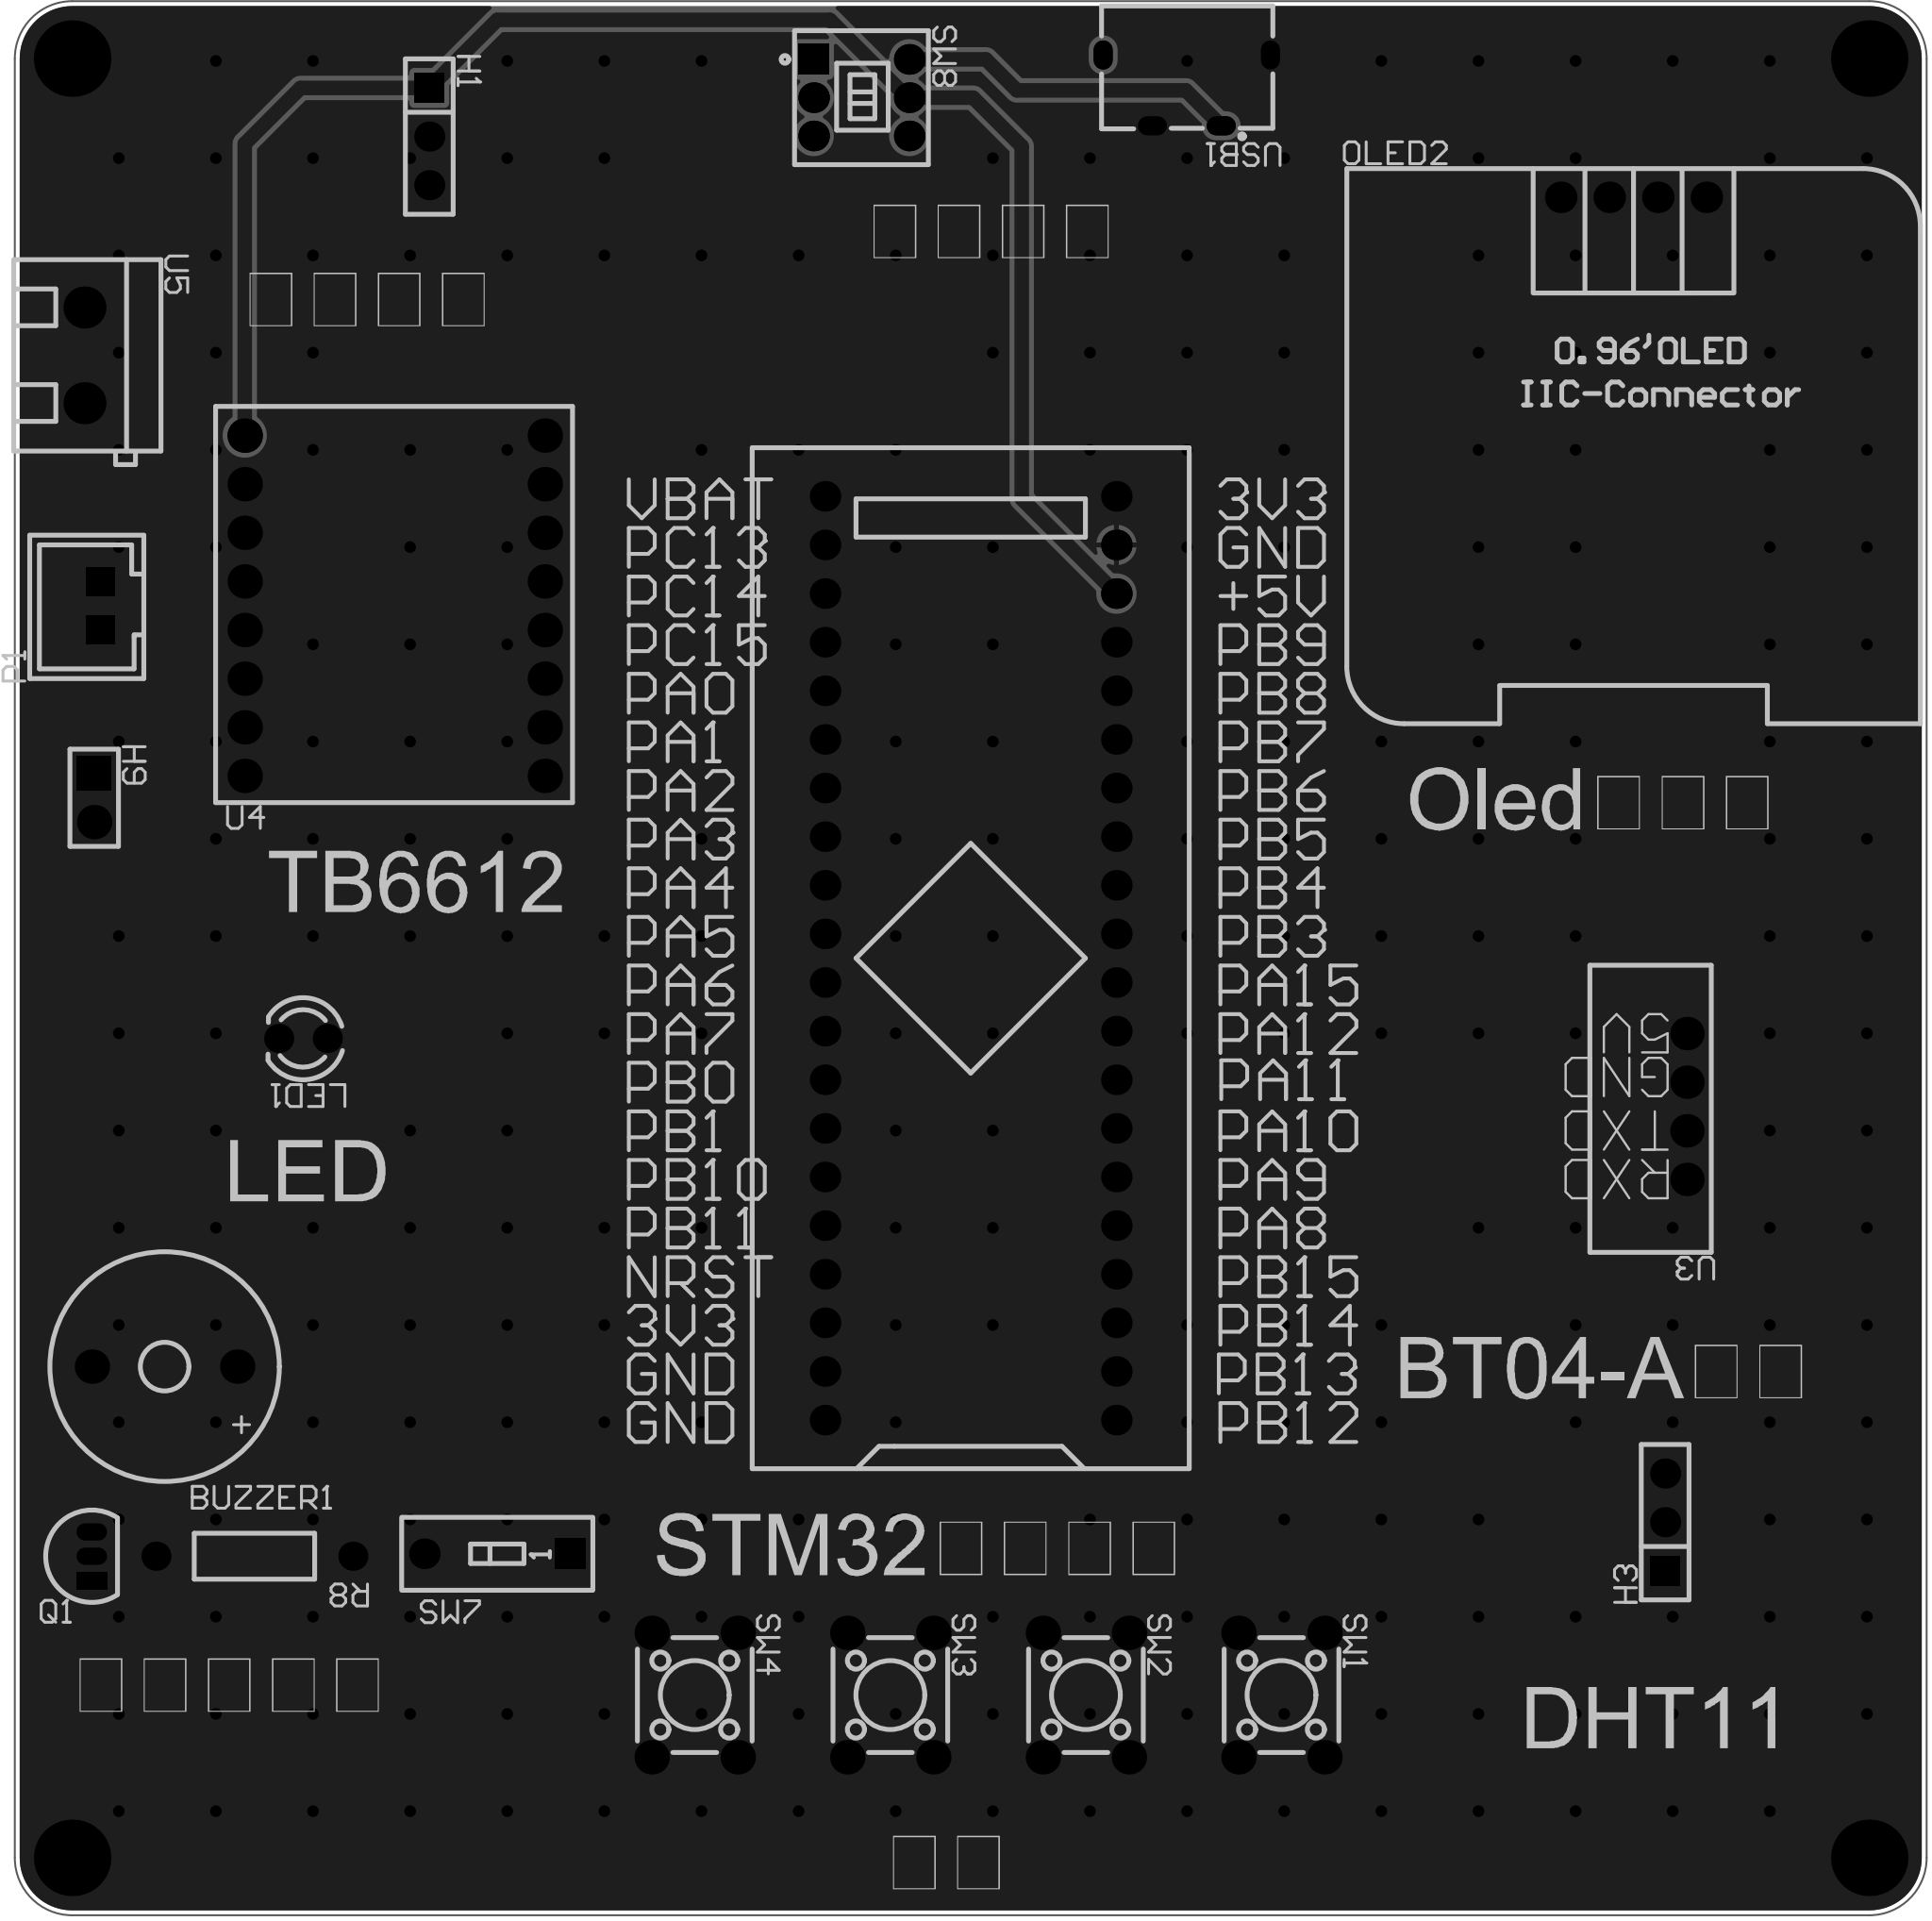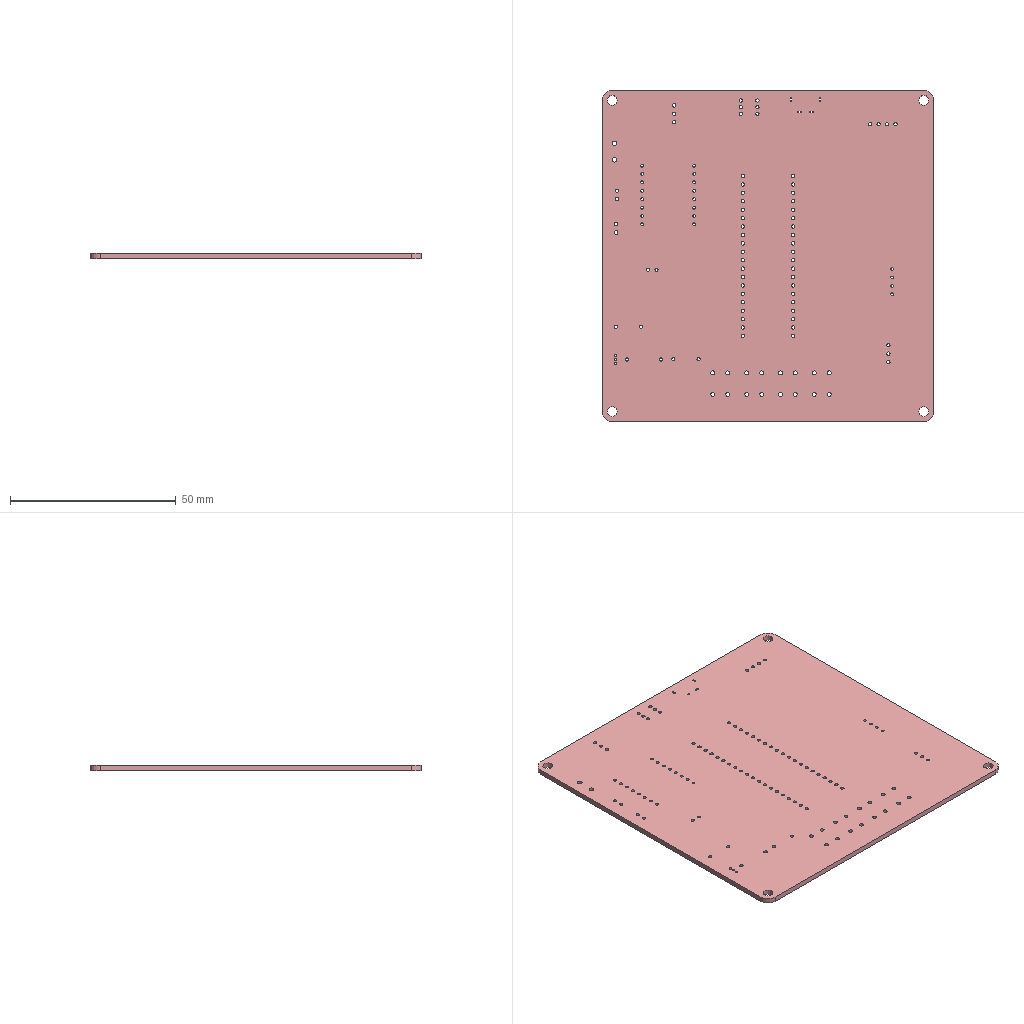Circuit board layout | Altium Designer | box 100 x 100 x 1.6 mm
Layer stack:
# Altium Designer layer stack of  (unit mm; dielectric type: 0 none, 1 core, 2 prepreg, 3 surface material)
index,name,kind,layer,copper_thickness_mm,dielectric_type,dielectric_thickness_mm,dielectric_material,dielectric_constant
0,Top Paste Mask Layer,other,,,,,,
1,Top Silkscreen Layer,other,,,,,,
2,Top Solder Mask Layer,dielectric,,,3,0.01,,3.3
3,Top Layer,copper,Top Layer,0.035,,,,
4,Dielectric1,dielectric,,,3,1.51,FR4,4.5
5,Bottom Layer,copper,Bottom Layer,0.035,,,,
6,Bottom Solder Mask Layer,dielectric,,,3,0.01,,3.3
7,Bottom Silkscreen Layer,other,,,,,,
8,Bottom Paste Mask Layer,other,,,,,,
# drill layer pairs: low layer,high layer
drill_pair,Top Layer,Bottom Layer
Part placement:
Designator,Comment,Layer,Footprint,Center-X(mm),Center-Y(mm),Rotation
U1,STM32F103C8T6-Card,TopLayer,CONN-TH_L53.3-W22.9_STM32F103C8T6-CARD,141.351,130.937,90
BUZZER1,2.3kHz,TopLayer,BUZ-TH_BD12.0-P7.60-D0.6-FD,99.187,109.601,180
H1,,TopLayer,HDR-TH_3P-P2.54-V-F,113.03,173.863,270
H3,,TopLayer,HDR-TH_3P-P2.54-V-F,177.673,101.473,90
H9,,TopLayer,HDR-TH_2P-P2.54-V-M-1,95.504,139.319,270
LED1,,TopLayer,LED_TH-3mm,106.426,126.746,180
OLED2,,TopLayer,0.96OLED_4P,176.022,170.688,0
P1,XH2.54直插座-2P,TopLayer,CONN-TH_XH2.54-2P,95.813,149.356,90
Q1,,TopLayer,S8050_TO_92,95.377,99.695,90
R8,10kΩ,TopLayer,Res_1/4W,103.886,99.695,180
SW1,,TopLayer,SW-TH_4P-L6.0-W6.0-P4.50-LS6.5,157.607,92.441,270
SW2,,TopLayer,SW-TH_4P-L6.0-W6.0-P4.50-LS6.5,147.377,92.441,270
SW3,,TopLayer,SW-TH_4P-L6.0-W6.0-P4.50-LS6.5,137.147,92.441,270
SW7,拨码开关1位,TopLayer,SW-TH_2P-L3.9-W9.9-P2.54-LS7.6,116.586,99.822,180
SW4,,TopLayer,SW-TH_4P-L6.0-W6.0-P4.50-LS6.5,126.917,92.441,270
SW8,TK-6700-1,TopLayer,SW-TH_TK-6700-1,135.636,175.895,270
U3,,TopLayer,BT04-A,178.816,123.19,180
U4,,TopLayer,tb6612,111.227,149.352,0
U5,KF301-5.0-2P,TopLayer,CONN-TH_P5.00_KF301-5.0-2P,94.996,162.433,270
USB1,KH-TYPE-C-2P,TopLayer,USB-SMD_KH-TYPE-C-2P,152.654,176.276,180
Pad and via stacks:
# Altium Designer via and pad stacks of  (unit mm). Each distinct definition once, with the count of objects using it.
# via: kind,start_layer,end_layer,hole_mm,diameter_mm,mode(0 simple;1 top-mid-bottom;2 full stack),diameter_per_layer,count,example_net
# pad: kind,layer,hole_mm,hole_type(0 round;1 square;2 slot),plating,top_size,top_shape(1 round;2 rect;3 octagon;9 rounded rect),mid_size,bottom_size,mode,footprint,size_per_layer,count,example
pad,Multi-Layer,3,0,plated,4x4,1,4x4,4x4,0,,,4,1
pad,Multi-Layer,1,0,plated,1.6x1.6,1,1.6x1.6,1.6x1.6,0,CONN-TH_L53.3-W22.9_STM32F103C8T6-CARD,,40,U1.1
pad,Multi-Layer,1,0,plated,1.8x1.8,1,1.8x1.8,1.8x1.8,0,BUZ-TH_BD12.0-P7.60-D0.6-FD,,2,BUZZER1.2
pad,Multi-Layer,1.02,0,plated,1.575x1.575,1,1.575x1.575,1.575x1.575,0,HDR-TH_3P-P2.54-V-F,,4,H1.3
pad,Multi-Layer,1.02,0,plated,1.575x1.575,2,1.575x1.575,1.575x1.575,0,HDR-TH_3P-P2.54-V-F,,2,H1.1
pad,Multi-Layer,1.1,0,plated,1.8x1.8,1,1.8x1.8,1.8x1.8,0,HDR-TH_2P-P2.54-V-M-1,,1,H9.2
pad,Multi-Layer,1.1,0,plated,1.8x1.8,2,1.8x1.8,1.8x1.8,0,HDR-TH_2P-P2.54-V-M-1,,1,H9.1
pad,Multi-Layer,0.9144,0,plated,1.524x1.524,1,1.524x1.524,1.524x1.524,0,LED_TH-3mm,,2,LED1.1
pad,Multi-Layer,1,0,plated,1.65x1.65,1,1.65x1.65,1.65x1.65,0,0.96OLED_4P,,4,OLED2.4
pad,Multi-Layer,1,2,plated,1.524x1.524,2,1.524x1.524,1.524x1.524,0,CONN-TH_XH2.54-2P,,2,P1.1
pad,Multi-Layer,0.701,0,plated,0.8992x1.6,2,0.8992x1.6,0.8992x1.6,0,S8050_TO_92,,1,Q1.1
pad,Multi-Layer,0.701,0,plated,0.8992x1.6,1,0.8992x1.6,0.8992x1.6,0,S8050_TO_92,,2,Q1.2
pad,Multi-Layer,1,0,plated,1.524x1.524,1,1.524x1.524,1.524x1.524,0,Res_1/4W,,2,R8.1
pad,Multi-Layer,1.2,0,plated,1.8x1.8,1,1.8x1.8,1.8x1.8,0,SW-TH_4P-L6.0-W6.0-P4.50-LS6.5,,16,SW1.1
pad,Multi-Layer,1,0,plated,1.6x1.6,2,1.6x1.6,1.6x1.6,0,SW-TH_2P-L3.9-W9.9-P2.54-LS7.6,,1,SW7.1
pad,Multi-Layer,1,0,plated,1.6x1.6,1,1.6x1.6,1.6x1.6,0,SW-TH_2P-L3.9-W9.9-P2.54-LS7.6,,1,SW7.2
pad,Multi-Layer,1,0,plated,1.6x1.6,2,1.6x1.6,1.6x1.6,0,SW-TH_TK-6700-1,,1,SW8.1
pad,Multi-Layer,1,0,plated,1.6x1.6,1,1.6x1.6,1.6x1.6,0,SW-TH_TK-6700-1,,5,SW8.2
pad,Multi-Layer,0.8,0,plated,1.75x1.75,1,1.75x1.75,1.75x1.75,0,BT04-A,,4,U3.1
pad,Multi-Layer,0.9,0,plated,1.8x1.8,1,1.8x1.8,1.8x1.8,0,tb6612,,16,U4.1
pad,Multi-Layer,1.4,0,plated,2.2x2.2,1,2.2x2.2,2.2x2.2,0,CONN-TH_P5.00_KF301-5.0-2P,,2,U5.1
pad,Multi-Layer,0.45,2,plated,1x1.524,1,1x1.524,1x1.524,0,USB-SMD_KH-TYPE-C-2P,,2,USB1.1
pad,Multi-Layer,0.5,2,plated,1x1.524,1,1x1.524,1x1.524,0,USB-SMD_KH-TYPE-C-2P,,2,USB1.3
via,Top Layer,Bottom Layer,0.3048,0.61,0,,271,GND
Copper pours:
name,layer,net,type(0 solid;1 hatched;2 none)
Bottom Layer-GND,Bottom Layer,GND,0
Top Layer-GND,Top Layer,GND,0
Design rules, without the lines most boards share:
# Altium Designer design rules of  (exported by Altium Designer, unit mm)
# columns: name | kind | enabled | priority | scope1 | scope2 | descriptor | typed fields (field=value)
Copper_copperRegion_copperThickness1oz | 0 | disabled | 4 | All | All | Clearance Constraint (Gap=5.984mil) (Disabled)(All),(All) | gap=0.152
Copper_copperRegion_copperThickness1oz_1 | 63 | disabled | 4 | All | All | Board Clearance Constraint (Gap=0mil) (Disabled)(All) |
Copper_copperRegion_Copper_copperRegion | 0 | disabled | 5 | All | All | Clearance Constraint (Gap=5.984mil) (Disabled)(All),(All) | gap=0.152
Copper_copperRegion_Copper_copperRegion_1 | 63 | disabled | 5 | All | All | Board Clearance Constraint (Gap=0mil) (Disabled)(All) |
copperThickness1oz | 0 | enabled | 6 | All | All | Clearance Constraint (Gap=5.984mil) (All),(All) | gap=0.152
copperThickness1oz_1 | 63 | enabled | 6 | All | All | Board Clearance Constraint (Gap=0mil) (All) |
copperRegion_copperThickness1oz | 20 | disabled | 1 | All | All | Polygon Connect Rule(Relief Connect )(Conductor Width=10mil) (Relief Angle=90 Angle) (Entries=4) (Air Gap Width=10mil) (Disabled)(All),(All) | connect_style(0=relief,1=direct,2=none)=0 relief_conductor_width=0.254 relief_entries=4
copperRegion_Copper_copperRegion | 20 | disabled | 2 | All | All | Polygon Connect Rule(Relief Connect )(Conductor Width=10mil) (Relief Angle=90 Angle) (Entries=4) (Air Gap Width=10mil) (Disabled)(All),(All) | connect_style(0=relief,1=direct,2=none)=0 relief_conductor_width=0.254 relief_entries=4
copperRegion | 20 | enabled | 3 | All | All | Polygon Connect Rule(Relief Connect )(Conductor Width=10mil) (Relief Angle=90 Angle) (Entries=4) (Air Gap Width=10mil) (All),(All) | connect_style(0=relief,1=direct,2=none)=0 relief_conductor_width=0.254 relief_entries=4